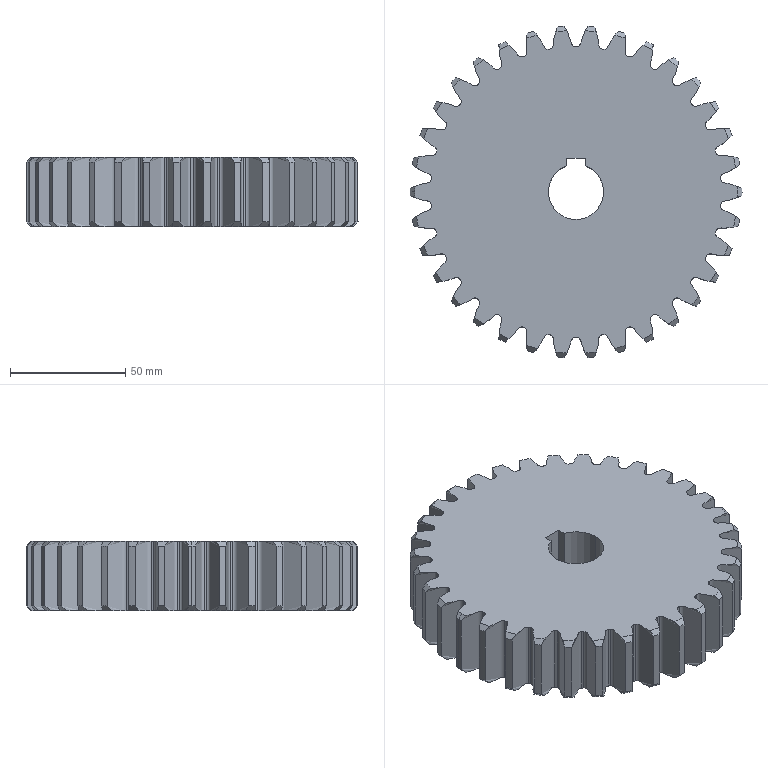Part | SolidWorks | features ICE 5, Chamfer 3, CirPattern 1, Extrusion 1, RefAxis 1 | 1 solid | 215 faces | box 144 x 143.631 x 30 mm | volume 417182 mm3 | cylinder 72 | cone 70 | spline 68 | plane 5 | commonest cylinder face diameters 144 x35 126 x34 24 x3